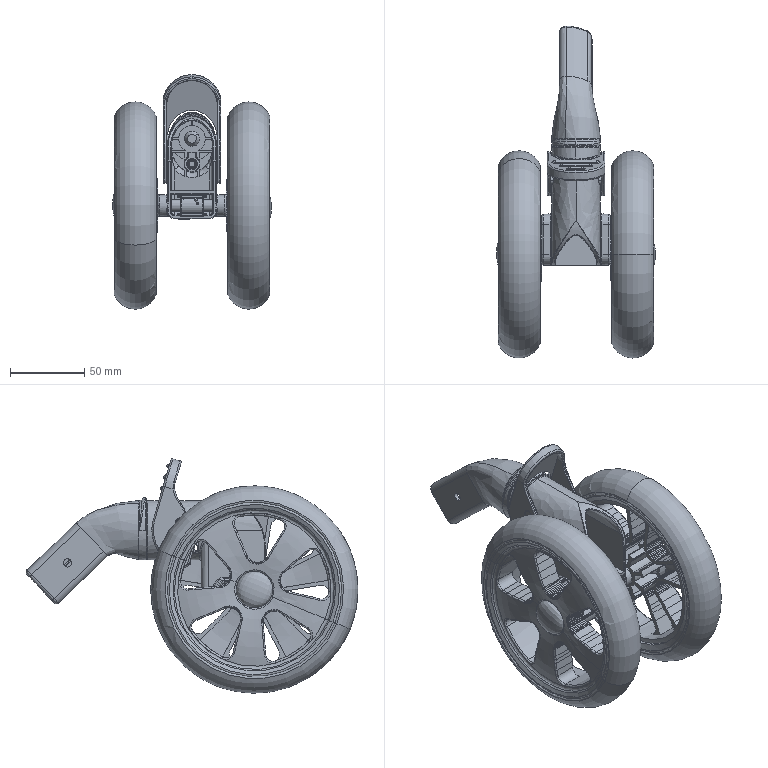Part | SolidWorks | 15 solids | 2392 faces | box 107.069 x 223.806 x 158.072 mm | volume 470883 mm3 | spline 1073 | cylinder 643 | plane 375 | torus 194 | cone 58 | sphere 49 | commonest cylinder face diameters 1 x113 0.6 x108 4 x42 2 x40 10 x39 7 x28